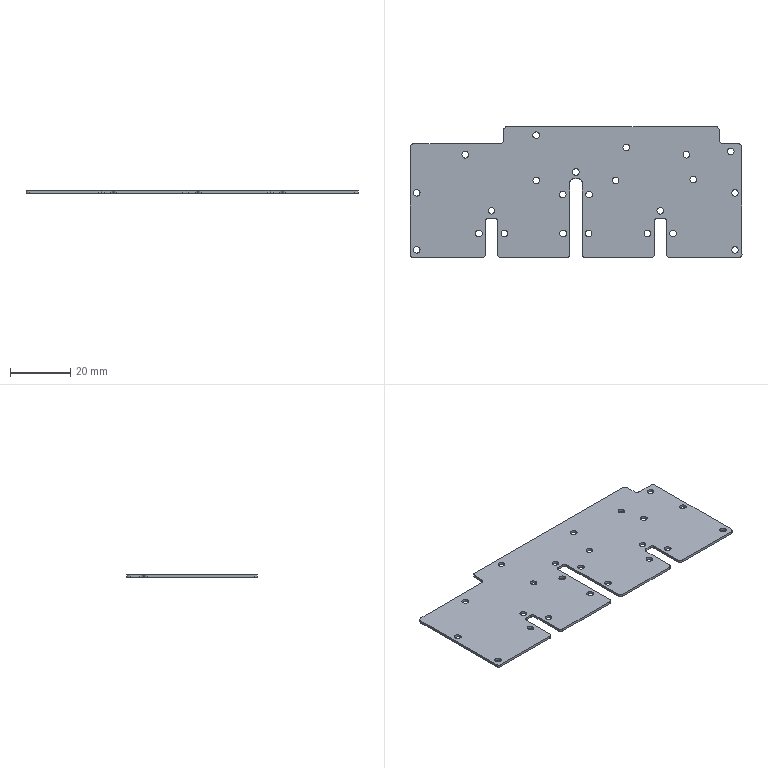Part | STEP file | 1 to 8 power divider PCB | 1 solid | 65 faces | box 110 x 43.34 x 0.832 mm | volume 3538 mm3 | cylinder 43 | plane 22 | commonest cylinder face diameters 2.2 x23 2 x14 2.54 x6